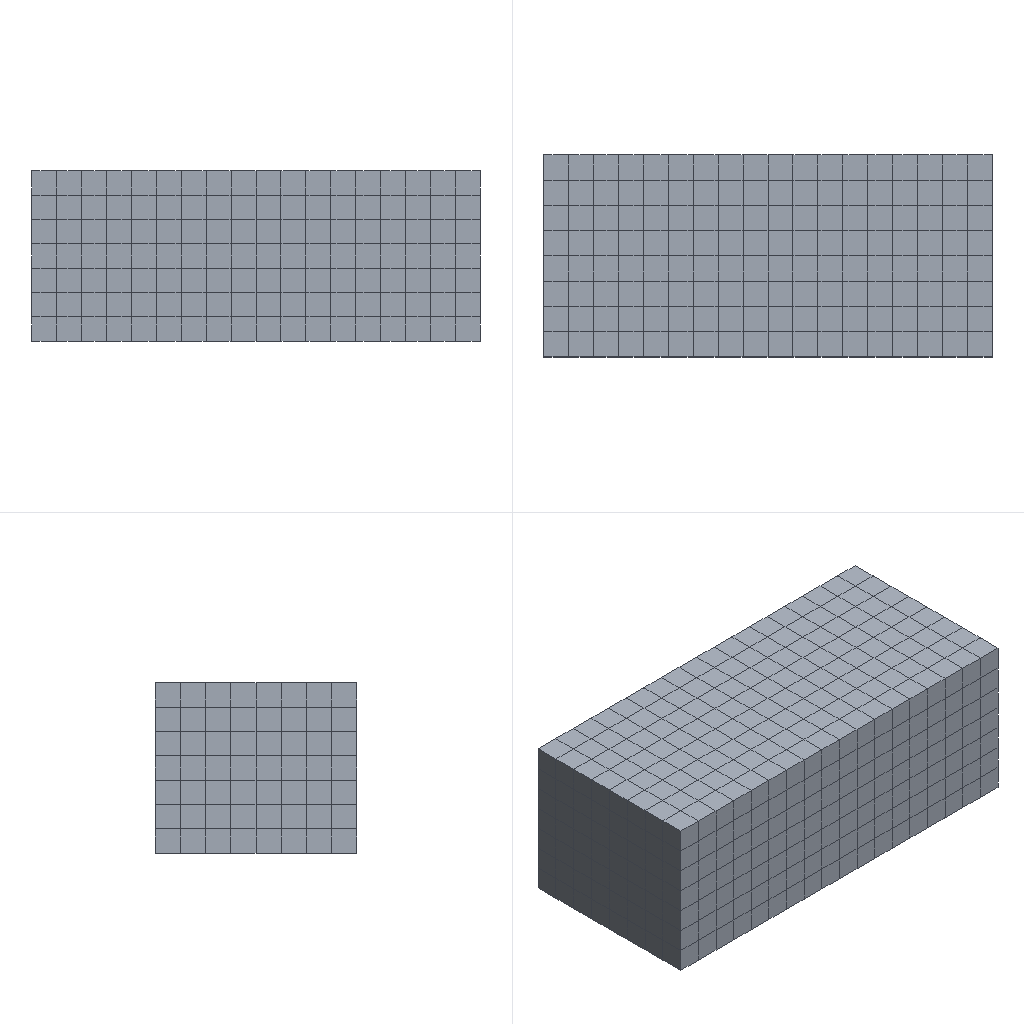Simulation study | abaqus
Set-up summary:
category,name,step,type,value,unit,region
solver,abaqus
solver,version,,,Abaqus/Standard 2020
units,not stated in the deck,,not stated
analysis,deck,,thermal,thermal
load_step,Step-1,Step-1,thermal
load_step,Step-2,Step-2,thermal
load_step,Step-3,Step-3,thermal
load_step,Step-4,Step-4,thermal
load_step,Step-5,Step-5,thermal
load_step,requested,,,5
mesh,nodes,,,1368
mesh,elements,,,1008
element_type,DC3D8,,solid,1008
load,load commands in deck,,count,8
bc,support commands in deck,,count,7
material,WORK,,in results
check,setup vs results,,match,"per instance, exact: element labels, types and connectivity; labels of the nodes the elements use; coordinates of those nodes at SINGLE_PRECISION in 1 of 1 instance(s)"
Abaqus input file, long lists of numbers shortened:
*Heading
** Job name: Job-1 Model name: Model-1
** Generated by: Abaqus/CAE 2020
*Preprint, echo=NO, model=NO, history=NO, contact=NO
**
** PARTS
**
*Part, name=Part-1
*Node
      1,           0.,        -450.,         380.
      2,           0.,      -393.75,         380.
** (1366 more lines like these left out)
*Element, type=DC3D8
   1,   73,   74,   83,   82,    1,    2,   11,   10
   2,   74,   75,   84,   83,    2,    3,   12,   11
** (1006 more lines like these left out)
*Nset, nset=Set-6, generate
    1,  1368,     1
*Elset, elset=Set-6, generate
    1,  1008,     1
** Section: Section-1
*Solid Section, elset=Set-6, material=work
,
*End Part
**
**
** ASSEMBLY
**
*Assembly, name=Assembly
**
*Instance, name=Part-1-1, part=Part-1
*End Instance
**
*Nset, nset=Set-3, instance=Part-1-1, generate
    1,  1368,     1
*Elset, elset=Set-3, instance=Part-1-1, generate
    1,  1008,     1
*Nset, nset=Set-4, instance=Part-1-1, generate
    1,  1368,     1
*Elset, elset=Set-4, instance=Part-1-1, generate
    1,  1008,     1
*Elset, elset=_Surf-18_S1, internal, instance=Part-1-1, generate
  953,  1008,     1
*Elset, elset=_Surf-18_S6, internal, instance=Part-1-1, generate
    1,  1001,     8
*Elset, elset=_Surf-18_S2, internal, instance=Part-1-1, generate
  1,  56,   1
*Elset, elset=_Surf-18_S4, internal, instance=Part-1-1, generate
    8,  1008,     8
*Elset, elset=_Surf-18_S3, internal, instance=Part-1-1
   1,   2,   3,   4,   5,   6,   7,   8,  57,  58,  59,  60,  61,  62,  63,  64
 113, 114, 115, 116, 117, 118, 119, 120, 169, 170, 171, 172, 173, 174, 175, 176
** (7 more lines like these left out)
*Elset, elset=_Surf-18_S5, internal, instance=Part-1-1
   49,   50,   51,   52,   53,   54,   55,   56,  105,  106,  107,  108,  109,  110,  111,  112
  161,  162,  163,  164,  165,  166,  167,  168,  217,  218,  219,  220,  221,  222,  223,  224
** (7 more lines like these left out)
*Surface, type=ELEMENT, name=Surf-18
_Surf-18_S1, S1
_Surf-18_S6, S6
_Surf-18_S2, S2
_Surf-18_S4, S4
_Surf-18_S3, S3
_Surf-18_S5, S5
*Elset, elset=_Surf-19_S1, internal, instance=Part-1-1, generate
  953,  1008,     1
*Elset, elset=_Surf-19_S6, internal, instance=Part-1-1, generate
    1,  1001,     8
*Elset, elset=_Surf-19_S2, internal, instance=Part-1-1, generate
  1,  56,   1
*Elset, elset=_Surf-19_S4, internal, instance=Part-1-1, generate
    8,  1008,     8
*Elset, elset=_Surf-19_S3, internal, instance=Part-1-1
   1,   2,   3,   4,   5,   6,   7,   8,  57,  58,  59,  60,  61,  62,  63,  64
 113, 114, 115, 116, 117, 118, 119, 120, 169, 170, 171, 172, 173, 174, 175, 176
** (7 more lines like these left out)
*Elset, elset=_Surf-19_S5, internal, instance=Part-1-1
   49,   50,   51,   52,   53,   54,   55,   56,  105,  106,  107,  108,  109,  110,  111,  112
  161,  162,  163,  164,  165,  166,  167,  168,  217,  218,  219,  220,  221,  222,  223,  224
** (7 more lines like these left out)
*Surface, type=ELEMENT, name=Surf-19
_Surf-19_S1, S1
_Surf-19_S6, S6
_Surf-19_S2, S2
_Surf-19_S4, S4
_Surf-19_S3, S3
_Surf-19_S5, S5
*Elset, elset=_Surf-20_S1, internal, instance=Part-1-1, generate
  953,  1008,     1
*Elset, elset=_Surf-20_S6, internal, instance=Part-1-1, generate
    1,  1001,     8
*Elset, elset=_Surf-20_S2, internal, instance=Part-1-1, generate
  1,  56,   1
*Elset, elset=_Surf-20_S4, internal, instance=Part-1-1, generate
    8,  1008,     8
*Elset, elset=_Surf-20_S3, internal, instance=Part-1-1
   1,   2,   3,   4,   5,   6,   7,   8,  57,  58,  59,  60,  61,  62,  63,  64
 113, 114, 115, 116, 117, 118, 119, 120, 169, 170, 171, 172, 173, 174, 175, 176
** (7 more lines like these left out)
*Elset, elset=_Surf-20_S5, internal, instance=Part-1-1
   49,   50,   51,   52,   53,   54,   55,   56,  105,  106,  107,  108,  109,  110,  111,  112
  161,  162,  163,  164,  165,  166,  167,  168,  217,  218,  219,  220,  221,  222,  223,  224
** (7 more lines like these left out)
*Surface, type=ELEMENT, name=Surf-20
_Surf-20_S1, S1
_Surf-20_S6, S6
_Surf-20_S2, S2
_Surf-20_S4, S4
_Surf-20_S3, S3
_Surf-20_S5, S5
*Elset, elset=_Surf-21_S1, internal, instance=Part-1-1, generate
  953,  1008,     1
*Elset, elset=_Surf-21_S6, internal, instance=Part-1-1, generate
    1,  1001,     8
*Elset, elset=_Surf-21_S2, internal, instance=Part-1-1, generate
  1,  56,   1
*Elset, elset=_Surf-21_S4, internal, instance=Part-1-1, generate
    8,  1008,     8
*Elset, elset=_Surf-21_S3, internal, instance=Part-1-1
   1,   2,   3,   4,   5,   6,   7,   8,  57,  58,  59,  60,  61,  62,  63,  64
 113, 114, 115, 116, 117, 118, 119, 120, 169, 170, 171, 172, 173, 174, 175, 176
** (7 more lines like these left out)
*Elset, elset=_Surf-21_S5, internal, instance=Part-1-1
   49,   50,   51,   52,   53,   54,   55,   56,  105,  106,  107,  108,  109,  110,  111,  112
  161,  162,  163,  164,  165,  166,  167,  168,  217,  218,  219,  220,  221,  222,  223,  224
** (7 more lines like these left out)
*Surface, type=ELEMENT, name=Surf-21
_Surf-21_S1, S1
_Surf-21_S6, S6
_Surf-21_S2, S2
_Surf-21_S4, S4
_Surf-21_S3, S3
_Surf-21_S5, S5
*Elset, elset=_Surf-22_S1, internal, instance=Part-1-1, generate
  953,  1008,     1
*Elset, elset=_Surf-22_S6, internal, instance=Part-1-1, generate
    1,  1001,     8
*Elset, elset=_Surf-22_S2, internal, instance=Part-1-1, generate
  1,  56,   1
*Elset, elset=_Surf-22_S4, internal, instance=Part-1-1, generate
    8,  1008,     8
*Elset, elset=_Surf-22_S3, internal, instance=Part-1-1
   1,   2,   3,   4,   5,   6,   7,   8,  57,  58,  59,  60,  61,  62,  63,  64
 113, 114, 115, 116, 117, 118, 119, 120, 169, 170, 171, 172, 173, 174, 175, 176
** (7 more lines like these left out)
*Elset, elset=_Surf-22_S5, internal, instance=Part-1-1
   49,   50,   51,   52,   53,   54,   55,   56,  105,  106,  107,  108,  109,  110,  111,  112
  161,  162,  163,  164,  165,  166,  167,  168,  217,  218,  219,  220,  221,  222,  223,  224
** (7 more lines like these left out)
*Surface, type=ELEMENT, name=Surf-22
_Surf-22_S1, S1
_Surf-22_S6, S6
_Surf-22_S2, S2
_Surf-22_S4, S4
_Surf-22_S3, S3
_Surf-22_S5, S5
*Elset, elset=_Surf-23_S1, internal, instance=Part-1-1, generate
  953,  1008,     1
*Elset, elset=_Surf-23_S6, internal, instance=Part-1-1, generate
    1,  1001,     8
*Elset, elset=_Surf-23_S2, internal, instance=Part-1-1, generate
  1,  56,   1
*Elset, elset=_Surf-23_S4, internal, instance=Part-1-1, generate
    8,  1008,     8
*Elset, elset=_Surf-23_S3, internal, instance=Part-1-1
   1,   2,   3,   4,   5,   6,   7,   8,  57,  58,  59,  60,  61,  62,  63,  64
 113, 114, 115, 116, 117, 118, 119, 120, 169, 170, 171, 172, 173, 174, 175, 176
** (7 more lines like these left out)
*Elset, elset=_Surf-23_S5, internal, instance=Part-1-1
   49,   50,   51,   52,   53,   54,   55,   56,  105,  106,  107,  108,  109,  110,  111,  112
  161,  162,  163,  164,  165,  166,  167,  168,  217,  218,  219,  220,  221,  222,  223,  224
** (7 more lines like these left out)
*Surface, type=ELEMENT, name=Surf-23
_Surf-23_S1, S1
_Surf-23_S6, S6
_Surf-23_S2, S2
_Surf-23_S4, S4
_Surf-23_S3, S3
_Surf-23_S5, S5
*Elset, elset=_Surf-24_S1, internal, instance=Part-1-1, generate
  953,  1008,     1
*Elset, elset=_Surf-24_S6, internal, instance=Part-1-1, generate
    1,  1001,     8
*Elset, elset=_Surf-24_S2, internal, instance=Part-1-1, generate
  1,  56,   1
*Elset, elset=_Surf-24_S4, internal, instance=Part-1-1, generate
    8,  1008,     8
*Elset, elset=_Surf-24_S3, internal, instance=Part-1-1
   1,   2,   3,   4,   5,   6,   7,   8,  57,  58,  59,  60,  61,  62,  63,  64
 113, 114, 115, 116, 117, 118, 119, 120, 169, 170, 171, 172, 173, 174, 175, 176
** (7 more lines like these left out)
*Elset, elset=_Surf-24_S5, internal, instance=Part-1-1
   49,   50,   51,   52,   53,   54,   55,   56,  105,  106,  107,  108,  109,  110,  111,  112
  161,  162,  163,  164,  165,  166,  167,  168,  217,  218,  219,  220,  221,  222,  223,  224
** (7 more lines like these left out)
*Surface, type=ELEMENT, name=Surf-24
_Surf-24_S1, S1
_Surf-24_S6, S6
_Surf-24_S2, S2
_Surf-24_S4, S4
_Surf-24_S3, S3
_Surf-24_S5, S5
*Elset, elset=_Surf-25_S1, internal, instance=Part-1-1, generate
  953,  1008,     1
*Elset, elset=_Surf-25_S6, internal, instance=Part-1-1, generate
    1,  1001,     8
*Elset, elset=_Surf-25_S2, internal, instance=Part-1-1, generate
  1,  56,   1
*Elset, elset=_Surf-25_S4, internal, instance=Part-1-1, generate
    8,  1008,     8
*Elset, elset=_Surf-25_S3, internal, instance=Part-1-1
   1,   2,   3,   4,   5,   6,   7,   8,  57,  58,  59,  60,  61,  62,  63,  64
 113, 114, 115, 116, 117, 118, 119, 120, 169, 170, 171, 172, 173, 174, 175, 176
** (7 more lines like these left out)
*Elset, elset=_Surf-25_S5, internal, instance=Part-1-1
   49,   50,   51,   52,   53,   54,   55,   56,  105,  106,  107,  108,  109,  110,  111,  112
  161,  162,  163,  164,  165,  166,  167,  168,  217,  218,  219,  220,  221,  222,  223,  224
** (7 more lines like these left out)
*Surface, type=ELEMENT, name=Surf-25
_Surf-25_S1, S1
_Surf-25_S6, S6
_Surf-25_S2, S2
_Surf-25_S4, S4
_Surf-25_S3, S3
_Surf-25_S5, S5
*Elset, elset=_Surf-26_S1, internal, instance=Part-1-1, generate
  953,  1008,     1
*Elset, elset=_Surf-26_S6, internal, instance=Part-1-1, generate
    1,  1001,     8
*Elset, elset=_Surf-26_S2, internal, instance=Part-1-1, generate
  1,  56,   1
*Elset, elset=_Surf-26_S4, internal, instance=Part-1-1, generate
    8,  1008,     8
*Elset, elset=_Surf-26_S3, internal, instance=Part-1-1
   1,   2,   3,   4,   5,   6,   7,   8,  57,  58,  59,  60,  61,  62,  63,  64
 113, 114, 115, 116, 117, 118, 119, 120, 169, 170, 171, 172, 173, 174, 175, 176
** (7 more lines like these left out)
*Elset, elset=_Surf-26_S5, internal, instance=Part-1-1
   49,   50,   51,   52,   53,   54,   55,   56,  105,  106,  107,  108,  109,  110,  111,  112
  161,  162,  163,  164,  165,  166,  167,  168,  217,  218,  219,  220,  221,  222,  223,  224
** (7 more lines like these left out)
*Surface, type=ELEMENT, name=Surf-26
_Surf-26_S1, S1
_Surf-26_S6, S6
_Surf-26_S2, S2
_Surf-26_S4, S4
_Surf-26_S3, S3
_Surf-26_S5, S5
*Elset, elset=_Surf-27_S1, internal, instance=Part-1-1, generate
  953,  1008,     1
*Elset, elset=_Surf-27_S6, internal, instance=Part-1-1, generate
    1,  1001,     8
*Elset, elset=_Surf-27_S2, internal, instance=Part-1-1, generate
  1,  56,   1
*Elset, elset=_Surf-27_S4, internal, instance=Part-1-1, generate
    8,  1008,     8
*Elset, elset=_Surf-27_S3, internal, instance=Part-1-1
   1,   2,   3,   4,   5,   6,   7,   8,  57,  58,  59,  60,  61,  62,  63,  64
 113, 114, 115, 116, 117, 118, 119, 120, 169, 170, 171, 172, 173, 174, 175, 176
** (7 more lines like these left out)
*Elset, elset=_Surf-27_S5, internal, instance=Part-1-1
   49,   50,   51,   52,   53,   54,   55,   56,  105,  106,  107,  108,  109,  110,  111,  112
  161,  162,  163,  164,  165,  166,  167,  168,  217,  218,  219,  220,  221,  222,  223,  224
** (7 more lines like these left out)
*Surface, type=ELEMENT, name=Surf-27
_Surf-27_S1, S1
_Surf-27_S6, S6
_Surf-27_S2, S2
_Surf-27_S4, S4
_Surf-27_S3, S3
_Surf-27_S5, S5
*End Assembly
*Amplitude, name=Amp-1
             1.,     203539.115,              2.,     198334.325,              3.,     193262.629,              4.,     188320.623
             5.,     183504.992,              6.,     178812.503,              7.,     174240.008,              8.,     169784.438
             9.,      165442.804,             10.,     161212.192,             11.,     157089.762,             12.,     153072.749
            13.,      149158.457,           13.33,     147888.833,             14.,      145344.259,             15.,     141627.596
            16.,     138005.973,             17.,     134476.96,             18.,     131038.189,             19.,     127687.352
            20.,     124422.202,             21.,     121240.546,             22.,     118140.249,             23.,     115119.232
            24.,     112175.466,             25.,     109306.977,             26.,     106511.839,             27.,     103788.177
            28.,     101134.162,           28.75,      99188.285,             29.,     98548.015,             30.,     96028.
         30.667,     94383.077,             31.,     93572.424,             32.,     91179.642,             33.,     88848.046
            34.,     86576.073,             35.,     84362.197,             36.,     82204.933,             37.,     80102.834
            38.,      78054.489,             39.,     76058.522,             40.,     74113.595,             41.,     72218.403
            42.,     70371.674,             43.,     68572.168,             44.,     66818.678,             45.,       65110.028
            46.,     63445.07,             47.,     61822.688,             48.,     60241.792,             49.,     58701.322
            50.,     57200.244,             51.,     55737.551,             52.,     54312.261,             53.,     52923.418
            54.,     51570.089,             55.,     50251.367,             56.,     48966.367,             57.,     47714.226
            58.,     46494.104,             59.,     45305.182,             60.,     44146.663,             61.,      43017.769
            62.,     41917.742,             63.,     40845.845,             64.,     39801.357,             65.,     38783.579
            66.,      37791.827,             67.,      36825.435,             68.,     35883.755,             69.,      34966.155
            70.,     34072.02,             71.,     33200.749,             72.,     32351.758,             73.,     31524.476
            74.,     30718.35,             75.,     29932.837,             76.,     29167.411,             77.,     28421.558
            78.,     27694.778,             79.,     26986.582,             80.,     26296.496,             81.,     25624.056
            82.,     24968.812,             83.,     24330.323,             84.,     23708.162,             85.,     23101.91
            86.,     22511.16,             87.,     21935.517,             88.,     21374.594,             89.,     20828.015
            90.,     20295.412,             91.,     19776.429,             92.,     19270.717,             93.,     18777.937
            94.,     18297.758,             95.,     17829.858,             96.,     17373.923,             97.,      16929.646
            98.,      16496.731,             99.,     16074.885,            100.,     15663.827,            101.,     15263.28
           102.,     14872.976,            103.,      14492.653,            104.,     14122.054,            105.,     13760.933
           106.,     13409.046
*Amplitude, name=Amp-2
             1.,     132300.425,              2.,     128917.311,              3.,     125620.709,              4.,     122408.405
             5.,     119278.245,              6.,     116228.127,              7.,     113256.005,              8.,     110359.885
             9.,     107537.823,             10.,     104787.925,             11.,     102108.345,             12.,     99497.287
            13.,     96952.997,           13.33,     88733.3,             14.,      87206.555,             15.,     84976.557
            16.,     82803.584,             17.,     80686.176,             18.,     78622.913,             19.,     76612.411
            20.,     74653.321,             21.,     72744.327,             22.,     70884.149,             23.,     69071.539
            24.,     67305.28,             25.,     65584.186,             26.,     63907.103,             27.,     62272.906
            28.,     60680.497,           28.75,     59512.971,             29.,     59128.809,             30.,     57616.8
         30.667,     56629.846,             31.,     51464.833,             32.,     50148.803,             33.,     48866.425
            34.,     47616.84,             35.,     46399.208,             36.,      45212.713,             37.,     44056.559
            38.,     42929.969,             39.,     41832.187,             40.,     40762.477,             41.,      39720.122
            42.,      38704.421,             43.,     37714.693,             44.,     36750.273,             45.,      35810.515
            46.,      34894.789,             47.,     34002.478,             48.,     33132.986,             49.,     32285.727
            50.,     31460.134,             51.,       30655.653,             52.,     29871.744,             53.,     29107.88
            54.,     28363.549,             55.,     27638.252,             56.,     26931.502,             57.,     26242.824
            58.,     25571.757,             59.,     24917.85,             60.,      24280.665,             61.,     23659.773
            62.,      23054.758,             63.,      22465.215,             64.,     21890.746,             65.,     21330.968
            66.,     20785.505,             67.,     20253.989,             68.,     19736.065,             69.,     19231.385
            70.,       18739.611,             71.,     18260.412,             72.,     17793.467,             73.,     17338.462
            74.,     16895.092,             75.,      16463.06,             76.,     16042.076,             77.,     15631.857
            78.,     15232.128,             79.,      14842.62,             80.,     14463.073,             81.,     14093.231
            82.,     13732.847,             83.,     13381.678,             84.,     13039.489,             85.,     12706.05
            86.,     12381.138,             87.,     12064.535,             88.,     11756.027,             89.,     11455.408
            90.,     11162.477,             91.,     10877.036,             92.,     10598.895,             93.,     10327.865
            94.,     10063.767,             95.,     9806.422,             96.,     9555.657,             97.,     9311.305
            98.,     9073.202,             99.,     8841.187,            100.,     8615.105,            101.,     8394.804
           102.,     8180.137,            103.,     7970.959,            104.,     7767.13,            105.,     7568.513
           106.,     7374.975
**
** MATERIALS
**
*Material, name=work
*Conductivity
    20.7, 244.
 21.702, 344.
 22.662, 444.
 23.622, 544.
 24.582, 644.
 25.542, 744.
 26.502, 844.
 27.462, 944.
 28.422,1044.
 29.382,1144.
 30.342,1244.
 31.302,1344.
*Density
 7.8e-09,
*Elastic
 175000., 0.3274,    100.
 175000., 0.3274,    200.
 175000., 0.3274,    300.
 175000., 0.3274,    400.
 175000., 0.3274,    499.
 172500., 0.3274,    500.
 137470., 0.3274,    600.
 102439., 0.3356,    700.
 67408.5, 0.3438,    800.
 32728.3, 0.352,    899.
  32378., 0.3521,    900.
  20000.,  0.3603,   1000.
  14542., 0.3685,   1100.
  12896., 0.3768,   1200.
  11954., 0.385,   1300.
 10961.7, 0.3886,   1344.
 10925.5, 0.4187,   1345.
*Expansion
 1.18276e-05, 100.
 1.28536e-05, 200.
 1.37901e-05, 300.
 1.46372e-05, 400.
 1.54581e-05, 499.
 1.61496e-05, 500.
 1.67178e-05, 600.
 1.69072e-05, 700.
 1.72861e-05, 800.
 2.23733e-05, 899.
  2.3457e-05, 900.
 2.86125e-05,1000.
 3.17815e-05,1100.
 3.44199e-05,1200.
 3.59217e-05,1300.
 3.70582e-05,1344.
 3.70582e-05,1345.
*Plastic
160.,  0.,800.
190., 0.1,800.
200., 0.2,800.
210., 0.3,800.
212., 0.4,800.
214., 0.5,800.
215., 0.6,800.
*Specific Heat
 5.73229e+08, 244.
 5.82749e+08, 344.
 5.92269e+08, 444.
 6.01789e+08, 544.
 6.11309e+08, 644.
 6.20829e+08, 744.
 6.30349e+08, 844.
 6.39869e+08, 944.
 6.49389e+08,1044.
 6.58909e+08,1144.
 6.68429e+08,1244.
 6.77949e+08,1344.
**
** PHYSICAL CONSTANTS
**
*Physical Constants, absolute zero=-273., stefan boltzmann=5.67e-08
**
** PREDEFINED FIELDS
**
** Name: Predefined Field-1   Type: Temperature
*Initial Conditions, type=TEMPERATURE
Set-4, 30.
** ----------------------------------------------------------------
**
** STEP: Step-1
**
*Step, name=Step-1, nlgeom=NO, inc=10000
*Heat Transfer, end=PERIOD, deltmx=1e+15, mxdem=1.
0.01, 106., 0.0001, 106.,
**
** LOADS
**
** Name: Load-1   Type: Surface heat flux
*Dsflux, amplitude=Amp-1
Surf-25, S, 0.01
**
** OUTPUT REQUESTS
**
*Restart, write, frequency=0
**
** FIELD OUTPUT: F-Output-1
**
*Output, field
*Node Output
NT, RFL
*Element Output, directions=YES
HFL, TEMP
*Radiation Output
FTEMP,
*Output, history, frequency=0
*End Step
** ----------------------------------------------------------------
**
** STEP: Step-2
**
*Step, name=Step-2, nlgeom=NO, inc=1000
*Heat Transfer, end=PERIOD, deltmx=1e+06, mxdem=1.
1., 16.25, 0.0001625, 16.25,
**
** LOADS
**
** Name: Load-1   Type: Surface heat flux
*Dsflux, op=NEW
**
** INTERACTIONS
**
** Interaction: Int-1
*Sfilm
Surf-18, F, 30., 0.04
** Interaction: Int-2
*Sradiate
Surf-19, R, 30., 0.7
**
** OUTPUT REQUESTS
**
*Restart, write, frequency=0
**
** FIELD OUTPUT: F-Output-1
**
*Output, field
*Node Output
NT, RFL
*Element Output, directions=YES
HFL, TEMP
*Radiation Output
FTEMP,
*Output, history, frequency=0
*End Step
** ----------------------------------------------------------------
**
** STEP: Step-3
**
*Step, name=Step-3, nlgeom=NO, inc=1000
*Heat Transfer, end=PERIOD, deltmx=1e+06, mxdem=1.
1., 27.5, 0.000275, 27.5,
**
** INTERACTIONS
**
** Interaction: Int-1
*Sfilm, op=NEW
** Interaction: Int-2
*Sradiate, op=NEW
** Interaction: Int-3
*Sfilm, op=NEW
Surf-20, F, 30., 0.002
** Interaction: Int-4
*Sradiate, op=NEW
Surf-21, R, 30., 0.1
**
** OUTPUT REQUESTS
**
*Restart, write, frequency=0
**
** FIELD OUTPUT: F-Output-1
**
*Output, field
*Node Output
NT, RFL
*Element Output, directions=YES
HFL, TEMP
*Radiation Output
FTEMP,
*Output, history, frequency=0
*End Step
** ----------------------------------------------------------------
**
** STEP: Step-4
**
*Step, name=Step-4, nlgeom=NO, inc=1000
*Heat Transfer, end=PERIOD, deltmx=1e+07, mxdem=1.
1., 55., 0.00055, 55.,
**
** INTERACTIONS
**
** Interaction: Int-3
*Sfilm, op=NEW
** Interaction: Int-4
*Sradiate, op=NEW
** Interaction: Int-5
*Sfilm, op=NEW
Surf-22, F, 30., 0.0011
** Interaction: Int-6
*Sradiate, op=NEW
Surf-23, R, 30., 0.1
**
** OUTPUT REQUESTS
**
*Restart, write, frequency=0
**
** FIELD OUTPUT: F-Output-1
**
*Output, field
*Node Output
NT, RFL
*Element Output, directions=YES
HFL, TEMP
*Radiation Output
FTEMP,
*Output, history, frequency=0
*End Step
** ----------------------------------------------------------------
**
** STEP: Step-5
**
*Step, name=Step-5, nlgeom=NO, inc=10000
*Heat Transfer, end=PERIOD, deltmx=1e+07, mxdem=1.
1., 1000., 0.01, 1000.,
**
** INTERACTIONS
**
** Interaction: Int-5
*Sfilm, op=NEW
** Interaction: Int-6
*Sradiate, op=NEW
** Interaction: Int-7
*Sradiate, op=NEW
Surf-24, R, 30., 0.1
**
** OUTPUT REQUESTS
**
*Restart, write, frequency=0
**
** FIELD OUTPUT: F-Output-1
**
*Output, field
*Node Output
NT, RFL
*Element Output, directions=YES
HFL, TEMP
*Radiation Output
FTEMP,
*Output, history, frequency=0
*End Step
Results summary:
result,step,,partial,increments=0 time=0.0/106.0
result,step,,partial,increments=0 time=0.0/16.25
result,step,,partial,increments=0 time=0.0/27.5
result,step,,partial,increments=0 time=0.0/55.0
result,step,,partial,increments=0 time=0.0/1000.0
result,analysis,,,"heat transfer, deltamx"
result,last_loadstep,,,5
result,primary field,,,NT11